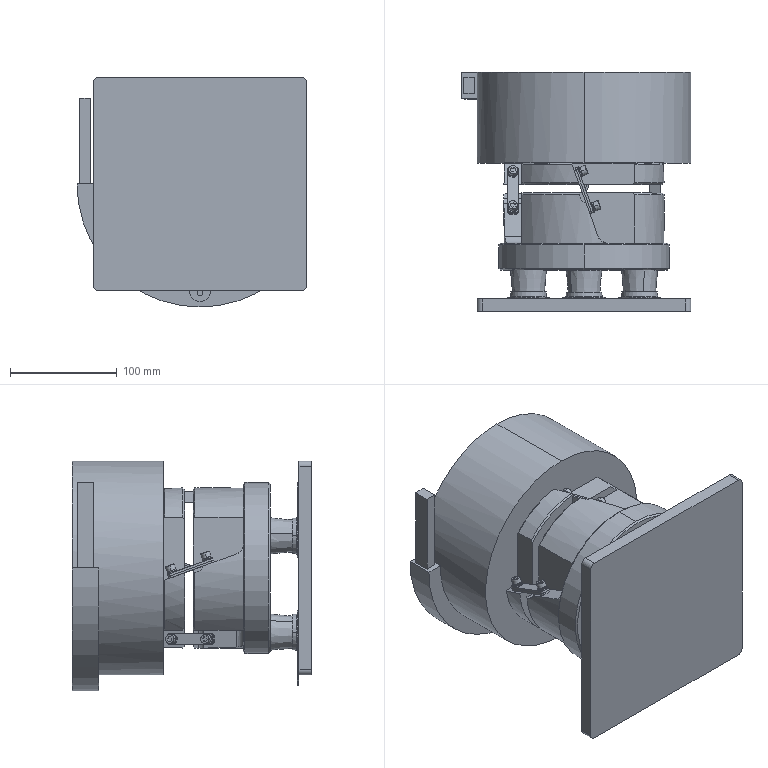Part | SolidWorks | features ReferencePattern 12, MirrorCompFeat 2 | 48 solids | 698 faces | box 215 x 224 x 215 mm | volume 2633576 mm3 | plane 272 | cylinder 245 | torus 108 | cone 73 | commonest cylinder face diameters 4 x32 6 x32 10 x20 5 x16 5.4 x16 5.5 x16